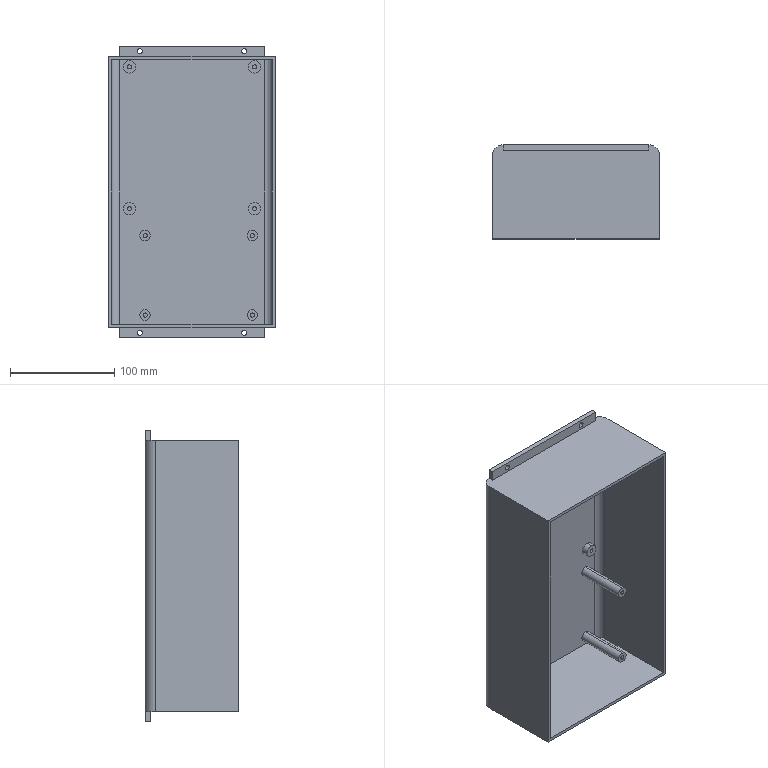Part | SolidWorks | features ICE 5, Extrusion 1, Fillet 1, Shell 1 | 1 solid | 79 faces | box 160 x 90 x 280 mm | volume 364305 mm3 | cylinder 44 | plane 35 | commonest cylinder face diameters 4 x16 5 x8 10 x8 12 x8 14 x2 20 x2